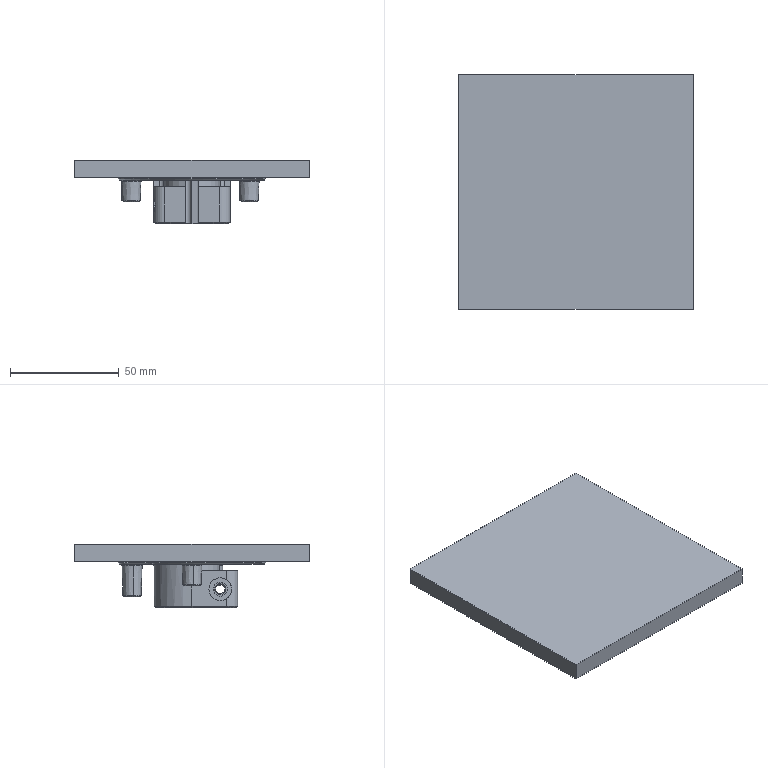NC program | NX | posted with a generic post | part box 108 x 108 x 29 mm
Lines 67 to 952 of 13118:
(ADAPTIVE_MILLING_COPY , TOOL : D10)
N108 T04 M6
N110 G54
N112 G17 G0 G90 X-44.769 Y1.065 S9500 M3
N114 G43 Z30. H4
N116 Z-11.5
N118 G94 G1 Z-12.5 F1000.
N120 X-43.298 Y0.606 F3500.
N122 G3 X-42.122 Y1.065 R1.017
N124 X-41.34 Y3.862 R6.974
N126 X-41.023 Y12.477 R84.168
N128 G1 X-41.017 Y14.102
N130 X-41.012 Y16.477
N132 X-41.009 Y20.602
N134 X-41.008 Y33.852
N136 X-41.006 Y34.102
N138 X-41.001 Y34.227
N140 G2 X-38.426 Y38.466 R5.818
N142 X-32.965 Y40.482 R12.575
N144 X-24.235 Y40.958 R63.696
N146 G1 X-22.985 Y40.968
N148 X-21.485 Y40.976
N150 X-19.485 Y40.981
N152 X-16.36 Y40.985
N154 X-8.86 Y40.986
N156 X34.015
N158 G2 X38.34 Y38.577 R5.654
N160 X40.446 Y33.155 R12.134
N162 X40.955 Y24.553 R60.117
N164 G1 X40.965 Y23.428
N166 X40.973 Y22.053
N168 X40.979 Y20.303
N170 X40.983 Y17.803
N172 X40.986 Y13.053
N174 Y-34.072
N176 G2 X38.627 Y-38.296 R5.658
N178 X33.219 Y-40.433 R11.969
N180 X25.368 Y-40.946 R53.229
N182 G1 X24.368 Y-40.957
N184 X23.118 Y-40.967
N186 X21.743 Y-40.975
N188 X19.868 Y-40.98
N190 X16.993 Y-40.984
N192 X10.993 Y-40.986
N194 X-34.007
N196 X-34.132 Y-40.984
N198 X-34.256 Y-40.978
N200 X-34.381 Y-40.968
N202 G2 X-38.554 Y-38.276 R5.918
N204 X-40.542 Y-32.542 R13.213
N206 X-40.963 Y-23.808 R71.53
N208 G1 X-40.971 Y-22.558
N210 X-40.978 Y-20.933
N212 X-40.982 Y-18.558
N214 X-40.985 Y-14.558
N216 X-40.986 Y-2.558
N218 X-40.985 Y-2.433
N220 G2 X-40.459 Y2.914 R75.914
N222 G3 X-40.036 Y14.777 R129.409
N224 G1 X-40.029 Y16.527
N226 X-40.023 Y19.027
N228 X-40.02 Y22.902
N230 X-40.019 Y30.902
N232 X-40.014 Y31.152
N234 X-40.001 Y31.402
N236 G2 X-36.211 Y37.401 R7.724
N238 X-29.72 Y39.501 R15.917
N240 X-20.487 Y39.945 R81.414
N242 G1 X-19.237 Y39.955
N244 X-17.862 Y39.963
N246 X-15.862 Y39.969
N248 X-12.862 Y39.973
N250 X-6.987 Y39.975
N252 X30.888 Y39.976
N254 G2 X37.258 Y36.398 R7.577
N256 X39.446 Y30.071 R15.247
N258 X39.939 Y21.091 R70.89
N260 G1 X39.948 Y20.216
N262 X39.957 Y18.841
N264 X39.965 Y17.091
N266 X39.971 Y14.716
N268 X39.974 Y11.091
N270 X39.975 Y1.841
N272 X39.976 Y-30.909
N274 X39.974 Y-31.034
N276 X39.971 Y-31.159
N278 X39.967 Y-31.284
N280 X39.96 Y-31.409
N282 X39.951 Y-31.533
N284 G2 X36.168 Y-37.406 R7.735
N286 X29.8 Y-39.487 R15.918
N288 X20.442 Y-39.945 R80.235
N290 G1 X19.192 Y-39.955
N292 X17.692 Y-39.963
N294 X15.817 Y-39.968
N296 X12.942 Y-39.973
N298 X7.442 Y-39.975
N300 X-30.933 Y-39.976
N302 G2 X-37.282 Y-36.358 R7.599
N304 X-39.437 Y-30.149 R15.163
N306 X-39.94 Y-21.045 R70.918
N308 X-39.936 Y-3.296 R812.597
N310 G1 X-39.919 Y-2.921
N312 X-39.898 Y-2.547
N314 X-39.875 Y-2.172
N316 X-39.84 Y-1.674
N318 X-39.802 Y-1.175
N320 X-39.75 Y-0.552
N322 X-39.662 Y0.444
N324 X-39.618 Y0.942
N326 X-39.555 Y1.689
N328 X-39.486 Y2.562
N330 X-39.421 Y3.434
N332 X-39.361 Y4.307
N334 X-39.319 Y4.931
N336 X-39.283 Y5.555
N338 G3 X-39.034 Y21.426 R343.319
N340 G2 X-38.975 Y29.424 R178.184
N342 X-34.302 Y36.408 R8.936
N344 X-27.281 Y38.497 R18.368
N346 X-17.421 Y38.936 R93.979
N348 G1 X-16.046 Y38.945
N350 X-14.296 Y38.953
N352 X-12.046 Y38.959
N354 X-8.671 Y38.963
N356 X-3.561 Y38.964
N358 G2 X3.303 Y39.046 R47.053
N360 G1 X4.053 Y39.032
N362 X4.803 Y39.021
N364 X5.678 Y39.012
N366 X6.927 Y39.003
N368 X8.427 Y38.996
N370 X10.552 Y38.991
N372 X14.052 Y38.988
N374 G2 X29.177 Y38.954 R866.28
N376 X36.409 Y34.261 R8.925
N378 X38.494 Y27.24 R18.348
N380 X38.94 Y16.754 R98.696
N382 G1 X38.949 Y15.254
N384 X38.956 Y13.379
N386 X38.961 Y10.754
N388 X38.964 Y6.504
N390 Y3.275
N392 X39.115 Y1.633
N394 X39.117 Y1.589
N396 G3 X38.987 Y-17.595 R936.994
N398 G2 X38.941 Y-29.344 R390.863
N400 X34.438 Y-36.303 R8.88
N402 X27.444 Y-38.466 R17.694
N404 X16.585 Y-38.941 R97.643
N406 G1 X15.21 Y-38.949
N408 X13.21 Y-38.956
N410 X10.335 Y-38.961
N412 X5.835 Y-38.964
N414 X3.571
N416 X0.149 Y-39.149
N418 G3 X-8.983 Y-38.991 R158.538
N420 G1 X-12.608 Y-38.988
N422 X-23.358 Y-38.986
N424 X-27.858
N426 X-28.233 Y-38.984
N428 X-28.608 Y-38.979
N430 X-28.733 Y-38.975
N432 G2 X-36.375 Y-34.321 R8.914
N434 X-38.452 Y-27.556 R17.831
N436 X-38.934 Y-17.448 R87.455
N438 X-38.906 Y-3.969 R441.58
N440 G1 X-39.049 Y-2.792
N442 X-39.053 Y-2.739
N444 X-39.133 Y1.12
N446 X-39.132 Y1.154
N448 X-38.829 Y4.994
N450 X-38.822 Y5.047
N452 G3 X-38.139 Y12.505 R41.064
N454 X-38.022 Y26.629 R819.327
N456 G2 X-32.581 Y35.416 R9.886
N458 X-25.287 Y37.474 R20.171
N460 X-13.802 Y37.931 R112.235
N462 G1 X-12.302 Y37.939
N464 X-10.177 Y37.946
N466 X-9.052 Y37.948
N468 X-8.927 Y37.953
N470 X-8.803 Y37.972
N472 X-8.682 Y38.002
N474 X-8.61 Y38.028
N476 X-8.552 Y38.058
N478 X-8.453 Y38.097
N480 X-6.975 Y38.52
N482 X-6.897 Y38.536
N484 X-3.55 Y38.966
N486 X-3.002 Y39.033
N488 X0.93 Y39.138
N490 X4.813 Y38.852
N492 X4.866 Y38.845
N494 G3 X13.438 Y38.044 R41.155
N496 G1 X14.313 Y38.032
N498 X15.313 Y38.022
N500 X16.563 Y38.013
N502 X18.188 Y38.006
N504 X20.438 Y38.001
N506 X24.188 Y37.998
N508 X25.063 Y37.997
N510 X25.813 Y37.992
N512 X26.188 Y37.988
N514 X26.438 Y37.982
N516 X26.813 Y37.97
N518 G2 X35.444 Y32.489 R9.863
N520 X37.435 Y25.56 R19.981
N522 X37.922 Y15.077 R95.064
N524 G1 X37.932 Y13.702
N526 X37.94 Y11.952
N528 X37.947 Y9.702
N530 X37.958 Y9.577
N532 X37.966 Y9.524
N534 X38.003 Y9.403
N536 X38.015 Y9.351
N538 X38.754 Y5.547
N540 X38.761 Y5.494
N542 X38.966 Y3.254
N544 G3 X40.465 Y2.481 R1.002
N546 X40.963 Y3.158 Z-12.457 R1.168
N548 G1 X41.377 Y4.219 Z-12.4
N550 X41.758 Y5.184
N552 X42.123 Y6.156
N554 X42.148 Y6.436
N556 G3 X41.651 Y13.908 R140.663
N558 G1 X40.345 Y26.971
N560 G3 X38.411 Y33.371 R17.994
N562 X35.222 Y37.859 R20.243
N564 X32.725 Y39.597 R8.373
N566 X28.317 Y40.867 R16.339
N568 G1 X27.699 Y40.928
N570 X27.079 Y40.97
N572 X10.511 Y41.593
N574 X10.302 Y41.575
N576 X10.099 Y41.522
N578 X8.302 Y40.797
N580 X7.646 Y40.535 Z-12.435
N582 X6.996 Y40.259 Z-12.471
N584 G3 X6.603 Y39.835 Z-12.5 R1.05
N586 X7.329 Y38.411 R1.003
N588 G2 X10.796 Y37.599 R27.087
N590 G3 X17.766 Y37.064 R40.155
N592 G2 X25.514 Y36.94 R260.471
N594 X34.354 Y31.071 R10.496
N596 X36.444 Y23.525 R21.452
N598 X36.928 Y12.977 R117.191
N600 G1 X37.972 Y9.506
N602 G3 X39.786 Y9.277 R1.001
N604 X39.942 Y9.904 Z-12.467 R1.311
N606 G1 X40.051 Y11.246 Z-12.4
N608 X40.222 Y13.403
N610 X40.151 Y15.898
N612 X40.027 Y18.391
N614 X39.921 Y19.634
N616 X39.798 Y20.876
N618 X39.54 Y23.153
N620 X39.265 Y25.428
N622 G3 X38.313 Y29.465 R25.254
N624 G1 X37.965 Y30.533
N626 X37.573 Y31.584
N628 G3 X35.429 Y34.928 R13.143
N630 X30.858 Y38.712 R15.568
N632 X28.027 Y39.595 R9.941
N634 G1 X27.04 Y39.72
N636 X13.613 Y40.866
N638 X13.367 Y40.853
N640 X13.131 Y40.787
N642 X11.381 Y40.03
N644 X10.766 Y39.769 Z-12.433
N646 X10.159 Y39.486 Z-12.467
N648 G3 X9.758 Y38.976 Z-12.5 R1.041
N650 X10.431 Y37.684 R1.004
N652 G1 X13.96 Y36.654
N654 G3 X20.552 Y36.095 R38.497
N656 G2 X25.778 Y35.687 R27.98
N658 X33.321 Y29.649 R11.08
N660 X35.399 Y22.097 R22.306
N662 X35.829 Y15.738 R89.307
N664 G1 X35.86 Y15.602
N666 X36.869 Y13.164
N668 X36.887 Y13.114
N670 X36.959 Y12.875
N672 G3 X38.679 Y12.516 R1.002
N674 X38.93 Y13.274 Z-12.459 R1.203
N676 G1 X39.031 Y14.455 Z-12.4
N678 X39.216 Y16.668
N680 X38.785 Y20.234
N682 X38.324 Y23.797
N684 G3 X36.704 Y29.584 R27.23
N686 X33.339 Y34.787 R18.107
N688 X31.419 Y36.548 R10.792
N690 X28.75 Y37.863 R10.882
N692 X24.529 Y38.918 R23.277
N694 G1 X15.941 Y40.181
N696 G3 X15.369 Y40.095 R1.05
N698 G1 X13.732 Y39.322
N700 X13.136 Y39.046 Z-12.433
N702 X12.551 Y38.747 Z-12.466
N704 G3 X12.163 Y38.199 Z-12.5 R1.039
N706 X12.759 Y36.999 R1.005
N708 X16.284 Y35.731 R25.683
N710 X21.993 Y35.093 R45.718
N712 G2 X28.929 Y32.556 R12.455
N714 X33.291 Y25.84 R13.866
N716 X34.599 Y18.345 R33.316
N718 G3 X35.364 Y16.793 R7.546
N720 G1 X35.387 Y16.745
N722 X35.865 Y15.59
N724 G3 X37.461 Y15.232 R1.003
N726 X37.804 Y16.061 Z-12.454 R1.16
N728 G1 X37.919 Y17.132 Z-12.4
N730 X38.135 Y19.154
N732 Y19.321
N734 X38.115 Y19.487
N736 X37.55 Y21.918
N738 X36.928 Y24.334
N740 G3 X35.7 Y28.056 R38.762
N742 X33.191 Y32.649 R23.789
N744 X28.262 Y36.563 R11.856
N746 X24.717 Y37.721 R23.031
N748 G1 X18.384 Y39.219
N750 G3 X17.71 Y39.142 R1.038
N752 G1 X16.155 Y38.373
N754 X15.562 Y38.085 Z-12.433
N756 X14.98 Y37.776 Z-12.466
N758 G3 X14.602 Y37.225 Z-12.5 R1.039
N760 X15.202 Y36.037 R1.005
N762 G2 X17.431 Y35.08 R118.44
N764 G3 X21.586 Y34.206 R31.534
N766 G2 X29.329 Y30.003 R12.757
N768 X32.751 Y22.72 R16.901
N770 G1 X33.172 Y20.767
N772 G2 X34.713 Y18.005 R40.084
N774 G3 X36.129 Y17.633 R1.004
N776 X36.597 Y18.421 Z-12.453 R1.045
N778 G1 X36.756 Y19.459 Z-12.4
N780 X36.916 Y20.467
N782 X37.055 Y21.477
N784 X37.029 Y21.694
N786 X36.963 Y21.902
N788 X34.087 Y28.149
N790 G3 X31.714 Y31.774 R15.52
N792 X29.705 Y33.993 R29.61
N794 X28.105 Y35.159 R8.527
N796 X24.095 Y36.803 R14.419
N798 G1 X20.519 Y37.632
N800 X20.286 Y37.631
N802 X18.288 Y37.39
N804 X17.604 Y37.312 Z-12.434
N806 X16.922 Y37.213 Z-12.469
N808 G3 X16.412 Y36.874 Z-12.5 R1.045
N810 X16.737 Y35.362 R1.003
N812 X21.447 Y33.375 R21.384
N814 G2 X30.804 Y24.522 R14.117
N816 G3 X31.336 Y23.466 R2.743
N818 G1 X33.223 Y20.668
N820 G3 X34.948 Y20.781 R1.002
N822 X35.01 Y21.577 Z-12.459 R1.203
N824 G1 X34.826 Y22.748 Z-12.4
N826 X34.5 Y24.768
N828 X34.388 Y25.014
N830 X32.46 Y28.083
N832 X30.512 Y31.14
N834 G3 X28.095 Y33.619 R9.937
N836 G1 X27.677 Y33.886
N838 X27.248 Y34.135
N840 X22.523 Y36.639
N842 G3 X21.896 Y36.743 R1.042
N844 G1 X20.106 Y36.455
N846 X19.436 Y36.352 Z-12.434
N848 X18.769 Y36.227 Z-12.468
N850 G3 X18.263 Y35.849 Z-12.5 R1.043
N852 X18.626 Y34.389 R1.004
N854 G2 X21.251 Y32.836 R22.97
N856 X26.273 Y29.155 R21.415
N858 G3 X28.827 Y26.488 R31.938
N860 G1 X31.145 Y23.701
N862 G3 X32.732 Y25.217 R-1.1
N864 G1 X22.271 Y34.765
N866 G3 X20.93 Y33.03 R-1.1
N868 G1 X22.922 Y31.736
N870 X22.965 Y31.705
N872 X25.987 Y29.279
N874 X26.027 Y29.244
N876 X27.275 Y28.017
N878 G3 X28.228 Y27.763 R1.014
N880 G1 X28.559 Y27.849
N882 X30.494 Y28.352 Z-12.4
N884 G2 X31.22 Y28.405 R1.316
N886 X31.775 Y28.017 R1.038
N888 G1 X34.833 Y23.677
N890 G2 X38.083 Y17.999 R40.572
N892 X39.669 Y14.271 R41.594
N894 X41.517 Y7.555 R54.883
N896 X41.973 Y4.262 R32.266
N898 G1 X42.26 Y0.836
N900 G2 X41.821 Y-0.078 R1.011
N902 G1 X41.616 Y-0.215
N904 X39.956 Y-1.33 Z-12.5
N906 X39.663 Y-1.526
N908 X39.38 Y-1.734
N910 G3 X39.078 Y-2.346 R1.038
N912 G1 X38.655 Y-6.198
N914 X38.646 Y-6.251
N916 G3 X38.068 Y-12.337 R30.009
N918 G1 X38.054 Y-12.962
N920 X38.043 Y-13.587
N922 X38.031 Y-14.462
N924 X38.021 Y-15.462
N926 X38.012 Y-16.712
N928 X38.006 Y-18.337
N930 X38.001 Y-20.712
N932 X37.997 Y-24.962
N934 X37.992 Y-25.712
N936 X37.986 Y-26.212
N938 X37.981 Y-26.462
N940 X37.967 Y-26.836
N942 X37.962 Y-26.961
N944 G2 X32.576 Y-35.395 R9.827
N946 X25.287 Y-37.468 R20.171
N948 X14.552 Y-37.926 R103.173
N950 G1 X13.052 Y-37.935
N952 X11.177 Y-37.943
N954 X9.552 Y-37.947
N956 X9.427 Y-37.955
N958 X9.389 Y-37.96
N960 X7.996 Y-38.323
N962 X7.943 Y-38.334
N964 X4.107 Y-38.933
N966 X4.054 Y-38.938
N968 X3.555 Y-38.965
N970 G3 X2.762 Y-40.495 R1.002
N972 X3.426 Y-40.966 Z-12.458 R1.189
N974 G1 X4.514 Y-41.391 Z-12.4
N976 X5.468 Y-41.771
N978 X6.431 Y-42.127
N980 X6.737 Y-42.147
N982 X25.407 Y-40.474
N984 G3 X30.296 Y-39.549 R25.942
N986 G1 X31.375 Y-39.235
N988 X32.44 Y-38.879
N990 G3 X35.87 Y-36.877 R13.157
N992 X38.884 Y-33.763 R13.999
N994 X40.558 Y-29.806 R10.814
N996 X40.959 Y-26.728 R18.503
N998 G1 X41.672 Y-10.166
N1000 X41.654 Y-9.951
N1002 X41.598 Y-9.743
N1004 X40.857 Y-7.942
N1006 X40.599 Y-7.304 Z-12.434
N1008 X40.323 Y-6.674 Z-12.469
N1010 G3 X39.859 Y-6.272 Z-12.5 R1.045
N1012 X38.49 Y-6.984 R1.003
N1014 X37.443 Y-11.798 R312.943
N1016 X37.034 Y-20.282 R67.017
N1018 G2 X36.863 Y-26.277 R60.227
N1020 X31.057 Y-34.364 R10.499
N1022 X23.633 Y-36.434 R21.497
N1024 X13.023 Y-36.912 R106.51
N1026 G3 X11.752 Y-37.343 R12.485
N1028 G1 X9.333 Y-37.974
N1030 G3 X9.191 Y-39.861 R1.001
N1032 G1 X9.492 Y-39.937 Z-12.484
N1034 X9.802 Y-39.962 Z-12.469
N1036 X11.175 Y-40.069 Z-12.4
N1038 X13.23 Y-40.224
N1040 X15.725 Y-40.154
N1042 X18.218 Y-40.03
N1044 X19.461 Y-39.924
N1046 X20.703 Y-39.8
N1048 X23.808 Y-39.452
N1050 X26.911 Y-39.081
N1052 G3 X33.224 Y-36.598 R15.541
N1054 X36.96 Y-33.624 R32.384
N1056 X38.139 Y-31.962 R6.204
N1058 X39.284 Y-29.201 R26.959
N1060 X39.7 Y-27.259 R10.376
N1062 X40.504 Y-19.181 R248.222
N1064 G1 X40.969 Y-13.393
N1066 X40.955 Y-13.147
N1068 X40.887 Y-12.91
N1070 X40.121 Y-11.172
N1072 X39.859 Y-10.563 Z-12.433
N1074 X39.574 Y-9.965 Z-12.466
N1076 G3 X39.046 Y-9.565 Z-12.5 R1.039
N1078 X37.787 Y-10.212 R1.004
N1080 X36.581 Y-14.283 R37.512
N1082 X36.064 Y-21.758 R50.547
N1084 G2 X35.286 Y-27.176 R16.689
N1086 X29.128 Y-33.577 R11.415
N1088 X21.395 Y-35.475 R24.047
N1090 X15.784 Y-35.838 R146.53
N1092 G1 X15.664 Y-35.872
N1094 X15.64 Y-35.88
N1096 X15.491 Y-35.953
N1098 X15.442 Y-35.975
N1100 X12.747 Y-36.976
N1102 G3 X12.427 Y-38.657 R1.002
N1104 X13.196 Y-38.927 Z-12.458 R1.188
N1106 G1 X14.357 Y-39.036 Z-12.4
N1108 X16.536 Y-39.234
N1110 X19.824 Y-38.835
N1112 X23.108 Y-38.413
N1114 G3 X28.291 Y-37.159 R31.722
N1116 G1 X29.979 Y-36.581
N1118 G3 X32.732 Y-35.02 R11.162
N1120 X35.472 Y-32.665 R26.379
N1122 X37.004 Y-30.552 R11.075
N1124 X38.402 Y-27.13 R11.965
N1126 X39.08 Y-23.453 R40.725
N1128 G1 X40.053 Y-16.25
N1130 G3 X39.974 Y-15.705 R1.057
N1132 G1 X39.211 Y-14.016
N1134 X38.943 Y-13.41 Z-12.433
N1136 X38.653 Y-12.815 Z-12.466
N1138 G3 X38.122 Y-12.419 Z-12.5 R1.039
N1140 X36.871 Y-13.068 R1.005
N1142 G2 X35.997 Y-15.331 R28.083
N1144 G3 X35.247 Y-20.01 R20.412
N1146 G2 X34.472 Y-25.315 R22.683
N1148 X28.037 Y-32.422 R11.809
N1150 X20.077 Y-34.435 R24.637
N1152 G3 X18.127 Y-34.659 R17.841
N1154 G1 X15.546 Y-35.926
N1156 G3 X15.192 Y-37.43 R1.003
N1158 X15.97 Y-37.829 Z-12.455 R1.051
N1160 G1 X17.059 Y-37.956 Z-12.4
N1162 X19.101 Y-38.195
N1164 X19.273 Y-38.196
N1166 X19.444 Y-38.176
N1168 X21.874 Y-37.611
N1170 X24.291 Y-36.989
N1172 G3 X28.012 Y-35.761 R38.762
N1174 X32.603 Y-33.251 R23.375
N1176 X35.655 Y-29.949 R12.762
N1178 X37.53 Y-26.046 R17.726
N1180 X38.101 Y-23.02 R13.143
N1182 G1 X38.374 Y-18.876
N1184 X38.372 Y-18.713
N1186 X38.164 Y-16.587
N1188 X38.098 Y-15.848 Z-12.437
N1190 X38.005 Y-15.112 Z-12.474
N1192 X37.903 Y-14.877 Z-12.487
N1194 X37.749 Y-14.671 Z-12.5
N1196 G3 X36.124 Y-14.979 R1.002
N1198 X34.784 Y-18.473 R19.963
N1200 G2 X33.857 Y-23.13 R112.974
N1202 X26.663 Y-31.435 R12.535
N1204 X20.799 Y-33.142 R24.415
N1206 G1 X18.976 Y-34.242
N1208 X18.078 Y-34.683
N1210 G3 X17.692 Y-36.142 R1.004
N1212 X18.471 Y-36.584 Z-12.454 R1.048
N1214 G1 X19.533 Y-36.74 Z-12.4
N1216 X20.543 Y-36.892
N1218 X21.556 Y-37.025
N1220 X21.77 Y-36.998
N1222 X21.975 Y-36.933
N1224 X28.222 Y-34.057
N1226 G3 X31.847 Y-31.684 R15.52
N1228 X34.009 Y-29.735 R32.201
N1230 X35.219 Y-28.067 R8.131
N1232 X36.806 Y-24.037 R14.19
N1234 G1 X37.476 Y-20.939
N1236 X37.493 Y-20.78
N1238 Y-20.62
N1240 X37.275 Y-18.606
N1242 X37.112 Y-17.192 Z-12.471
N1244 G3 X36.82 Y-16.704 Z-12.5 R1.053
N1246 X35.226 Y-17.042 R1.003
N1248 G1 X34.189 Y-19.095
N1250 G2 X32.606 Y-23.439 R81.878
N1252 X24.744 Y-30.718 R13.939
N1254 G1 X24.511 Y-30.809
N1256 X24.394 Y-30.854
N1258 X24.159 Y-30.94
N1260 X23.924 Y-31.024
N1262 X23.806 Y-31.066
N1264 X23.693 Y-31.119
N1266 X23.625 Y-31.158
N1268 G2 X20.62 Y-33.221 R22.272
N1270 G3 X20.807 Y-35.01 R1.001
N1272 X21.509 Y-35.024 Z-12.464 R1.275
N1274 G1 X22.779 Y-34.812 Z-12.4
N1276 X24.642 Y-34.5
N1278 X24.808 Y-34.453
N1280 X24.967 Y-34.386
N1282 X26.597 Y-33.471
N1284 X28.206 Y-32.517
N1286 X29.725 Y-31.514
N1288 X31.212 Y-30.465
N1290 G3 X33.278 Y-28.493 R12.123
N1292 G1 X33.711 Y-27.887
N1294 X34.095 Y-27.25
N1296 X36.753 Y-22.312
N1298 G3 X36.858 Y-21.671 R1.041
N1300 G1 X36.557 Y-19.893
N1302 X36.45 Y-19.232 Z-12.433
N1304 X36.32 Y-18.576 Z-12.467
N1306 G3 X35.919 Y-18.065 Z-12.5 R1.041
N1308 X34.503 Y-18.415 R1.004
N1310 G2 X30.666 Y-24.621 R50.701
N1312 X28.294 Y-27.057 R17.902
N1314 G1 X25.475 Y-29.726
N1316 X25.434 Y-29.761
N1318 X23.555 Y-31.212
N1320 G3 X25.034 Y-32.83 R-1.1
N1322 G1 X34.837 Y-22.237
N1324 G3 X33.129 Y-20.859 R-1.1
N1326 G1 X30.9 Y-24.037
N1328 X30.867 Y-24.079
N1330 X28.336 Y-27.013
N1332 G3 X28.117 Y-27.887 R1.015
N1334 G1 X28.193 Y-28.22
N1336 X28.634 Y-30.171 Z-12.4
N1338 X28.707 Y-30.492
N1340 X28.727 Y-30.82
N1342 G2 X28.336 Y-31.513 R1.026
N1344 G1 X26.545 Y-32.869
N1346 X24.726 Y-34.187
N1348 G2 X16.91 Y-38.601 R54.397
N1350 X13.186 Y-40.036 R36.483
N1352 G1 X9.484 Y-41.212
N1354 G2 X4.092 Y-42.084 R23.67
N1356 G1 X0.948 Y-42.221
N1358 G2 X-0.004 Y-41.66 R1.055
N1360 G1 X-1.11 Y-39.993 Z-12.5
N1362 X-1.543 Y-39.362
N1364 G3 X-2.234 Y-39.039 R1.027
N1366 G1 X-3.754 Y-38.968
N1368 X-3.807 Y-38.963
N1370 G3 X-10.509 Y-38.136 R65.31
N1372 X-26.383 Y-37.984 R507.68
N1374 G2 X-35.475 Y-32.427 R9.907
N1376 X-37.488 Y-25.119 R20.565
N1378 X-37.928 Y-14.383 R107.531
N1380 G1 X-37.937 Y-12.883
N1382 X-37.944 Y-11.008
N1384 X-37.947 Y-9.633
N1386 X-37.949 Y-9.508
N1388 X-37.954 Y-9.45
N1390 G2 X-38.917 Y-3.881 R33.447
N1392 G3 X-40.365 Y-3.111 R1.002
N1394 X-40.912 Y-3.816 Z-12.454 R1.163
N1396 G1 X-41.31 Y-4.822 Z-12.4
N1398 X-41.7 Y-5.798
N1400 X-42.073 Y-6.781
N1402 X-42.099 Y-7.063
N1404 G3 X-41.602 Y-14.535 R140.663
N1406 G1 X-40.42 Y-26.354
N1408 G3 X-37.909 Y-34.112 R18.883
N1410 X-35.651 Y-37.445 R30.236
N1412 X-33.298 Y-39.372 R8.294
N1414 X-29.549 Y-40.62 R9.847
N1416 X-23.333 Y-41.129 R74.302
N1418 G1 X-10.829 Y-41.577
N1420 X-10.619 Y-41.558
N1422 X-10.416 Y-41.503
N1424 X-8.587 Y-40.758
N1426 X-7.952 Y-40.504 Z-12.434
N1428 X-7.325 Y-40.23 Z-12.468
N1430 G3 X-6.92 Y-39.76 Z-12.5 R1.044
N1432 X-7.647 Y-38.395 R1.003
N1434 X-12.208 Y-37.37 R38.848
N1436 X-20.697 Y-37.03 R82.243
N1438 G2 X-26.44 Y-36.842 R50.229
N1440 X-34.382 Y-31.024 R10.485
N1442 X-36.421 Y-23.719 R21.337
N1444 X-36.914 Y-12.986 R103.673
N1446 G1 X-36.935 Y-12.849
N1448 X-37.723 Y-10.468
N1450 X-37.737 Y-10.417
N1452 X-37.956 Y-9.441
N1454 G3 X-39.882 Y-9.348 R1.001
N1456 G1 X-39.942 Y-9.707 Z-12.482
N1458 X-39.965 Y-10.071 Z-12.464
N1460 X-40.061 Y-11.338 Z-12.4
N1462 X-40.206 Y-13.338
N1464 X-40.135 Y-15.833
N1466 X-40.011 Y-18.326
N1468 X-39.905 Y-19.569
N1470 X-39.782 Y-20.811
N1472 X-39.524 Y-23.088
N1474 X-39.249 Y-25.363
N1476 G3 X-37.665 Y-31.158 R25.856
N1478 X-36.075 Y-33.961 R15.325
N1480 X-33.523 Y-37.078 R27.793
N1482 X-31.855 Y-38.248 R6.295
N1484 X-29.088 Y-39.376 R25.214
N1486 X-27.14 Y-39.749 R9.417
N1488 G1 X-13.911 Y-40.8
N1490 X-13.672 Y-40.787
N1492 X-13.441 Y-40.724
N1494 X-11.679 Y-39.974
N1496 X-11.055 Y-39.714 Z-12.434
N1498 X-10.44 Y-39.433 Z-12.468
N1500 G3 X-10.038 Y-38.94 Z-12.5 R1.042
N1502 X-10.729 Y-37.618 R1.004
N1504 G2 X-13.284 Y-36.797 R28.082
N1506 G3 X-19.609 Y-36.12 R29.402
N1508 G2 X-25.22 Y-35.799 R44.307
N1510 X-33.348 Y-29.602 R11.081
N1512 X-35.419 Y-21.918 R22.602
N1514 X-35.839 Y-15.685 R105.077
N1516 X-36.946 Y-12.814 R24.239
N1518 G3 X-38.694 Y-12.526 R1.002
N1520 X-38.909 Y-13.231 Z-12.463 R1.223
N1522 G1 X-39.02 Y-14.476 Z-12.4
N1524 X-39.204 Y-16.605
N1526 X-38.805 Y-19.892
N1528 X-38.383 Y-23.175
N1530 G3 X-36.897 Y-29.007 R30.811
N1532 X-34.123 Y-33.706 R16.422
N1534 G1 X-33.379 Y-34.588
N1536 X-32.597 Y-35.436
N1538 G3 X-27.078 Y-38.441 R11.398
N1540 X-23.397 Y-39.095 R48.606
N1542 G1 X-16.106 Y-40.087
N1544 G3 X-15.552 Y-40.004 R1.054
N1546 G1 X-13.887 Y-39.234
N1548 X-13.287 Y-38.963 Z-12.433
N1550 X-12.698 Y-38.669 Z-12.466
N1552 G3 X-12.306 Y-38.126 Z-12.5 R1.039
N1554 X-12.924 Y-36.905 R1.005
N1556 X-16.605 Y-35.682 R29.14
N1558 X-22.069 Y-35.09 R49.043
N1560 G2 X-28.989 Y-32.514 R12.387
N1562 X-33.349 Y-25.653 R13.978
N1564 X-34.594 Y-18.399 R33.923
N1566 G3 X-34.928 Y-17.682 R3.229
N1568 G1 X-35.895 Y-15.513
N1570 G3 X-37.451 Y-15.153 R1.003
N1572 X-37.824 Y-15.999 Z-12.452 R1.142
N1574 G1 X-37.939 Y-17.039 Z-12.4
N1576 X-38.165 Y-19.073
N1578 Y-19.242
N1580 X-38.145 Y-19.41
N1582 X-37.58 Y-21.84
N1584 X-36.958 Y-24.257
N1586 G3 X-35.731 Y-27.979 R38.762
N1588 X-33.222 Y-32.572 R23.893
N1590 X-28.306 Y-36.508 R12.009
N1592 X-24.771 Y-37.695 R23.191
N1594 G1 X-18.346 Y-39.275
N1596 G3 X-17.657 Y-39.196 R1.032
N1598 G1 X-16.125 Y-38.423
N1600 X-15.535 Y-38.132 Z-12.433
N1602 X-14.956 Y-37.818 Z-12.466
N1604 G3 X-14.583 Y-37.262 Z-12.5 R1.039
N1606 X-15.164 Y-36.093 R1.005
N1608 X-20.049 Y-34.472 R14.029
N1610 G2 X-25.343 Y-33.056 R19.334
N1612 X-31.632 Y-26.228 R12.825
N1614 X-33.147 Y-20.824 R26.432
N1616 G1 X-33.173 Y-20.759
N1618 X-34.723 Y-18.046
N1620 G3 X-36.584 Y-18.423 R1.001
N1622 G1 X-36.574 Y-18.726 Z-12.485
N1624 X-36.517 Y-19.024 Z-12.47
N1626 X-36.254 Y-20.391 Z-12.4
N1628 X-35.892 Y-22.298
N1630 X-35.888 Y-22.968
N1632 X-35.845 Y-23.637
N1634 X-35.715 Y-24.246
N1636 X-35.544 Y-24.845
N1638 G3 X-34.653 Y-27.17 R14.826
N1640 G1 X-33.306 Y-29.904
N1642 G3 X-30.577 Y-33.307 R12.426
N1644 X-24.679 Y-36.648 R14.731
N1646 G1 X-23.474 Y-36.959
N1648 X-20.687 Y-37.563
N1650 X-20.525 Y-37.58
N1652 X-20.361 Y-37.579
N1654 X-18.353 Y-37.349
N1656 X-17.657 Y-37.273 Z-12.435
N1658 X-16.963 Y-37.179 Z-12.47
N1660 G3 X-16.464 Y-36.864 Z-12.5 R1.048
N1662 X-16.79 Y-35.313 R1.003
N1664 X-21.881 Y-33.236 R28.943
N1666 G2 X-30.834 Y-24.451 R14.09
N1668 G1 X-30.878 Y-24.334
N1670 X-30.963 Y-24.099
N1672 X-31.047 Y-23.863
N1674 X-31.098 Y-23.749
N1676 X-31.122 Y-23.703
N1678 G2 X-33.182 Y-20.743 R51.699
N1680 G3 X-34.978 Y-20.867 R1.001
N1682 X-35.005 Y-21.595 Z-12.463 R1.233
N1684 G1 X-34.798 Y-22.838 Z-12.4
N1686 X-34.455 Y-24.852
N1688 X-34.347 Y-25.09
N1690 X-31.916 Y-28.965
N1692 G3 X-28.957 Y-32.703 R28.094
N1694 X-25.472 Y-35.224 R13.022
N1696 G1 X-22.608 Y-36.638
N1698 G3 X-22.008 Y-36.729 R1.046
N1700 G1 X-20.184 Y-36.437
N1702 X-19.525 Y-36.337 Z-12.433
N1704 X-18.87 Y-36.214 Z-12.467
N1706 G3 X-18.352 Y-35.813 Z-12.5 R1.04
N1708 X-18.711 Y-34.388 R1.004
N1710 G2 X-24.171 Y-30.984 R114.75
N1712 X-27.175 Y-28.122 R15.653
N1714 G1 X-28.084 Y-27.274
N1716 X-28.121 Y-27.236
N1718 X-30.681 Y-24.317
N1720 X-30.714 Y-24.275
N1722 X-31.149 Y-23.664
N1724 G3 X-32.805 Y-25.098 R-1.1
N1726 G1 X-23.45 Y-34.039
N1728 G3 X-22.069 Y-32.335 R-1.1
N1730 G1 X-22.113 Y-32.305
N1732 X-25.204 Y-29.956
N1734 X-25.245 Y-29.922
N1736 X-27.256 Y-28.047
N1738 G3 X-28.181 Y-27.808 R1.014
N1740 G1 X-28.5 Y-27.888
N1742 X-30.44 Y-28.375 Z-12.4
N1744 X-30.734 Y-28.446
N1746 X-31.037 Y-28.464
N1748 G2 X-31.756 Y-28.047 R1.024
N1750 G1 X-34.632 Y-23.959
N1752 G2 X-37.062 Y-20.088 R63.788
N1754 X-38.822 Y-16.335 R29.36
N1756 G1 X-40.197 Y-12.715
N1758 G2 X-41.718 Y-6.167 R32.925
N1760 X-42.237 Y-0.579 R61.098
N1762 G1 X-42.453 Y4.273
N1764 G2 X-41.634 Y5.301 R1.005
N1766 G1 X-41.319 Y5.359
N1768 X-39.352 Y5.718 Z-12.5
N1770 G3 X-38.556 Y6.523 R1.01
N1772 G2 X-37.644 Y10.695 R36.404
N1774 G3 X-37.115 Y17.917 R44.776
N1776 G2 X-36.985 Y25.54 R252.887
N1778 X-31.093 Y34.369 R10.526
N1780 X-23.544 Y36.448 R21.468
N1782 X-11.934 Y36.917 R116.137
N1784 G3 X-10.442 Y37.015 R6.868
N1786 G2 X-8.573 Y38.047 R28.203
N1788 G3 X-8.236 Y39.539 R1.004
N1790 X-9.026 Y39.94 Z-12.454 R1.049
N1792 G1 X-10.105 Y40.053 Z-12.4
N1794 X-12.47 Y40.297
N1796 X-16.634 Y40.284
N1798 G3 X-21.808 Y39.822 R42.008
N1800 G1 X-23.846 Y39.509
N1802 X-25.881 Y39.18
N1804 G3 X-31.522 Y37.614 R32.855
N1806 X-35.474 Y35.27 R14.324
N1808 X-39.404 Y29.079 R12.504
N1810 G1 X-39.577 Y28.302
N1812 X-39.704 Y27.516
N1814 G3 X-40.461 Y20.063 R150.026
N1816 G1 X-40.966 Y13.268
N1818 X-40.952 Y13.028
N1820 X-40.887 Y12.797
N1822 X-40.129 Y11.04
N1824 X-39.868 Y10.425 Z-12.433
N1826 X-39.586 Y9.818 Z-12.467
N1828 G3 X-39.075 Y9.416 Z-12.5 R1.041
N1830 X-37.784 Y10.086 R1.004
N1832 X-36.615 Y14.324 R57.779
N1834 X-36.112 Y21.801 R52.761
N1836 G2 X-35.318 Y27.216 R16.61
N1838 X-29.25 Y33.543 R11.384
N1840 X-21.524 Y35.465 R23.975
N1842 X-12.537 Y35.917 R142.514
N1844 G3 X-11.254 Y36.267 R2.167
N1846 G1 X-11.178 Y36.342
N1848 X-10.108 Y37.205
N1850 G3 X-9.874 Y38.489 R1.005
N1852 X-10.776 Y38.999 Z-12.446 R1.107
N1854 G1 X-11.685 Y39.13 Z-12.4
N1856 X-12.844 Y39.303
N1858 X-14.006 Y39.455
N1860 X-15.254
N1862 X-16.501 Y39.404
N1864 X-17.121 Y39.335
N1866 X-17.739 Y39.25
N1868 X-24.562 Y38.112
N1870 G3 X-30.438 Y36.396 R26.088
N1872 G1 X-32.029 Y35.702